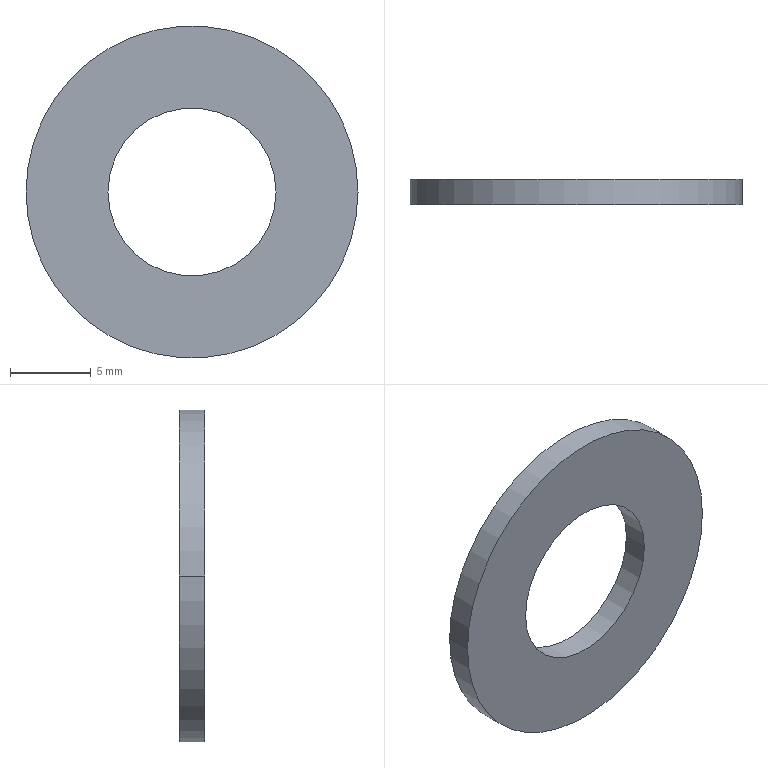Part | NX | features BREP 1 | 1 solid | 6 faces | box 20.574 x 1.575 x 20.574 mm | volume 389.406 mm3 | cylinder 4 | plane 2 | commonest cylinder face diameters 10.414 x2 20.574 x2
STEP:
#1=CARTESIAN_POINT('',(-10.287,0.,0.));
#2=VERTEX_POINT('',#1);
#3=CARTESIAN_POINT('',(10.287,0.,0.));
#4=VERTEX_POINT('',#3);
#5=CARTESIAN_POINT('',(0.,0.,0.));
#6=DIRECTION('',(0.,1.,0.));
#7=DIRECTION('',(-1.,0.,0.));
#8=AXIS2_PLACEMENT_3D('',#5,#6,#7);
#9=CIRCLE('',#8,10.287);
#10=EDGE_CURVE('',#2,#4,#9,.T.);
#11=ORIENTED_EDGE('',*,*,#10,.F.);
#12=CARTESIAN_POINT('',(0.,0.,0.));
#13=DIRECTION('',(0.,1.,0.));
#14=DIRECTION('',(1.,0.,0.));
#15=AXIS2_PLACEMENT_3D('',#12,#13,#14);
#16=CIRCLE('',#15,10.287);
#17=EDGE_CURVE('',#4,#2,#16,.T.);
#18=ORIENTED_EDGE('',*,*,#17,.F.);
#19=EDGE_LOOP('',(#11,#18));
#20=FACE_BOUND('',#19,.T.);
#21=CARTESIAN_POINT('',(-5.207,0.,0.));
#22=VERTEX_POINT('',#21);
#23=CARTESIAN_POINT('',(5.207,0.,0.));
#24=VERTEX_POINT('',#23);
#25=CARTESIAN_POINT('',(0.,0.,0.));
#26=DIRECTION('',(0.,-1.,0.));
#27=DIRECTION('',(-1.,0.,0.));
#28=AXIS2_PLACEMENT_3D('',#25,#26,#27);
#29=CIRCLE('',#28,5.207);
#30=EDGE_CURVE('',#22,#24,#29,.T.);
#31=ORIENTED_EDGE('',*,*,#30,.F.);
#32=CARTESIAN_POINT('',(0.,0.,0.));
#33=DIRECTION('',(0.,-1.,0.));
#34=DIRECTION('',(1.,0.,0.));
#35=AXIS2_PLACEMENT_3D('',#32,#33,#34);
#36=CIRCLE('',#35,5.207);
#37=EDGE_CURVE('',#24,#22,#36,.T.);
#38=ORIENTED_EDGE('',*,*,#37,.F.);
#39=EDGE_LOOP('',(#31,#38));
#40=FACE_BOUND('',#39,.T.);
#41=CARTESIAN_POINT('',(0.,0.,0.));
#42=DIRECTION('',(0.,1.,0.));
#43=DIRECTION('',(1.,0.,0.));
#44=AXIS2_PLACEMENT_3D('',#41,#42,#43);
#45=PLANE('',#44);
#46=ADVANCED_FACE('',(#20,#40),#45,.F.);
#47=CARTESIAN_POINT('',(-10.287,1.575,0.));
#48=VERTEX_POINT('',#47);
#49=CARTESIAN_POINT('',(-10.287,0.,0.));
#50=DIRECTION('',(0.,1.,0.));
#51=VECTOR('',#50,1000.);
#52=LINE('',#49,#51);
#53=EDGE_CURVE('',#2,#48,#52,.T.);
#54=ORIENTED_EDGE('',*,*,#53,.T.);
#55=CARTESIAN_POINT('',(10.287,1.575,0.));
#56=VERTEX_POINT('',#55);
#57=CARTESIAN_POINT('',(0.,1.575,0.));
#58=DIRECTION('',(0.,1.,0.));
#59=DIRECTION('',(1.,0.,0.));
#60=AXIS2_PLACEMENT_3D('',#57,#58,#59);
#61=CIRCLE('',#60,10.287);
#62=EDGE_CURVE('',#56,#48,#61,.T.);
#63=ORIENTED_EDGE('',*,*,#62,.F.);
#64=CARTESIAN_POINT('',(10.287,0.,0.));
#65=DIRECTION('',(0.,1.,0.));
#66=VECTOR('',#65,1000.);
#67=LINE('',#64,#66);
#68=EDGE_CURVE('',#4,#56,#67,.T.);
#69=ORIENTED_EDGE('',*,*,#68,.F.);
#70=ORIENTED_EDGE('',*,*,#17,.T.);
#71=EDGE_LOOP('',(#54,#63,#69,#70));
#72=FACE_BOUND('',#71,.T.);
#73=CARTESIAN_POINT('',(0.,0.,0.));
#74=DIRECTION('',(0.,1.,0.));
#75=DIRECTION('',(1.,0.,0.));
#76=AXIS2_PLACEMENT_3D('',#73,#74,#75);
#77=CYLINDRICAL_SURFACE('',#76,10.287);
#78=ADVANCED_FACE('',(#72),#77,.T.);
#79=ORIENTED_EDGE('',*,*,#68,.T.);
#80=CARTESIAN_POINT('',(0.,1.575,0.));
#81=DIRECTION('',(0.,1.,0.));
#82=DIRECTION('',(-1.,0.,0.));
#83=AXIS2_PLACEMENT_3D('',#80,#81,#82);
#84=CIRCLE('',#83,10.287);
#85=EDGE_CURVE('',#48,#56,#84,.T.);
#86=ORIENTED_EDGE('',*,*,#85,.F.);
#87=ORIENTED_EDGE('',*,*,#53,.F.);
#88=ORIENTED_EDGE('',*,*,#10,.T.);
#89=EDGE_LOOP('',(#79,#86,#87,#88));
#90=FACE_BOUND('',#89,.T.);
#91=CARTESIAN_POINT('',(0.,0.,0.));
#92=DIRECTION('',(0.,1.,0.));
#93=DIRECTION('',(1.,0.,0.));
#94=AXIS2_PLACEMENT_3D('',#91,#92,#93);
#95=CYLINDRICAL_SURFACE('',#94,10.287);
#96=ADVANCED_FACE('',(#90),#95,.T.);
#97=ORIENTED_EDGE('',*,*,#85,.T.);
#98=ORIENTED_EDGE('',*,*,#62,.T.);
#99=EDGE_LOOP('',(#97,#98));
#100=FACE_BOUND('',#99,.T.);
#101=CARTESIAN_POINT('',(-5.207,1.575,0.));
#102=VERTEX_POINT('',#101);
#103=CARTESIAN_POINT('',(5.207,1.575,0.));
#104=VERTEX_POINT('',#103);
#105=CARTESIAN_POINT('',(0.,1.575,0.));
#106=DIRECTION('',(0.,-1.,0.));
#107=DIRECTION('',(-1.,0.,0.));
#108=AXIS2_PLACEMENT_3D('',#105,#106,#107);
#109=CIRCLE('',#108,5.207);
#110=EDGE_CURVE('',#102,#104,#109,.T.);
#111=ORIENTED_EDGE('',*,*,#110,.T.);
#112=CARTESIAN_POINT('',(0.,1.575,0.));
#113=DIRECTION('',(0.,-1.,0.));
#114=DIRECTION('',(1.,0.,0.));
#115=AXIS2_PLACEMENT_3D('',#112,#113,#114);
#116=CIRCLE('',#115,5.207);
#117=EDGE_CURVE('',#104,#102,#116,.T.);
#118=ORIENTED_EDGE('',*,*,#117,.T.);
#119=EDGE_LOOP('',(#111,#118));
#120=FACE_BOUND('',#119,.T.);
#121=CARTESIAN_POINT('',(0.,1.575,0.));
#122=DIRECTION('',(0.,1.,0.));
#123=DIRECTION('',(1.,0.,0.));
#124=AXIS2_PLACEMENT_3D('',#121,#122,#123);
#125=PLANE('',#124);
#126=ADVANCED_FACE('',(#100,#120),#125,.T.);
#127=CARTESIAN_POINT('',(-5.207,0.,0.));
#128=DIRECTION('',(0.,1.,0.));
#129=VECTOR('',#128,1000.);
#130=LINE('',#127,#129);
#131=EDGE_CURVE('',#22,#102,#130,.T.);
#132=ORIENTED_EDGE('',*,*,#131,.T.);
#133=ORIENTED_EDGE('',*,*,#117,.F.);
#134=CARTESIAN_POINT('',(5.207,0.,0.));
#135=DIRECTION('',(0.,1.,0.));
#136=VECTOR('',#135,1000.);
#137=LINE('',#134,#136);
#138=EDGE_CURVE('',#24,#104,#137,.T.);
#139=ORIENTED_EDGE('',*,*,#138,.F.);
#140=ORIENTED_EDGE('',*,*,#37,.T.);
#141=EDGE_LOOP('',(#132,#133,#139,#140));
#142=FACE_BOUND('',#141,.T.);
#143=CARTESIAN_POINT('',(0.,0.,0.));
#144=DIRECTION('',(0.,1.,0.));
#145=DIRECTION('',(1.,0.,0.));
#146=AXIS2_PLACEMENT_3D('',#143,#144,#145);
#147=CYLINDRICAL_SURFACE('',#146,5.207);
#148=ADVANCED_FACE('',(#142),#147,.F.);
#149=ORIENTED_EDGE('',*,*,#138,.T.);
#150=ORIENTED_EDGE('',*,*,#110,.F.);
#151=ORIENTED_EDGE('',*,*,#131,.F.);
#152=ORIENTED_EDGE('',*,*,#30,.T.);
#153=EDGE_LOOP('',(#149,#150,#151,#152));
#154=FACE_BOUND('',#153,.T.);
#155=CARTESIAN_POINT('',(0.,0.,0.));
#156=DIRECTION('',(0.,1.,0.));
#157=DIRECTION('',(1.,0.,0.));
#158=AXIS2_PLACEMENT_3D('',#155,#156,#157);
#159=CYLINDRICAL_SURFACE('',#158,5.207);
#160=ADVANCED_FACE('',(#154),#159,.F.);
#161=CLOSED_SHELL('',(#46,#78,#96,#126,#148,#160));
#162=MANIFOLD_SOLID_BREP('',#161);
#163=(LENGTH_UNIT()NAMED_UNIT(*)SI_UNIT(.MILLI.,.METRE.));
#164=UNCERTAINTY_MEASURE_WITH_UNIT(LENGTH_MEASURE(0.00001),#163,'','');
#165=(NAMED_UNIT(*)PLANE_ANGLE_UNIT()SI_UNIT($,.RADIAN.));
#166=(NAMED_UNIT(*)SI_UNIT($,.STERADIAN.)SOLID_ANGLE_UNIT());
#167=(GEOMETRIC_REPRESENTATION_CONTEXT(3)GLOBAL_UNCERTAINTY_ASSIGNED_CONTEXT((#164))GLOBAL_UNIT_ASSIGNED_CONTEXT((#163,#165,#166))REPRESENTATION_CONTEXT('',''));
#168=ADVANCED_BREP_SHAPE_REPRESENTATION('',(#162),#167);